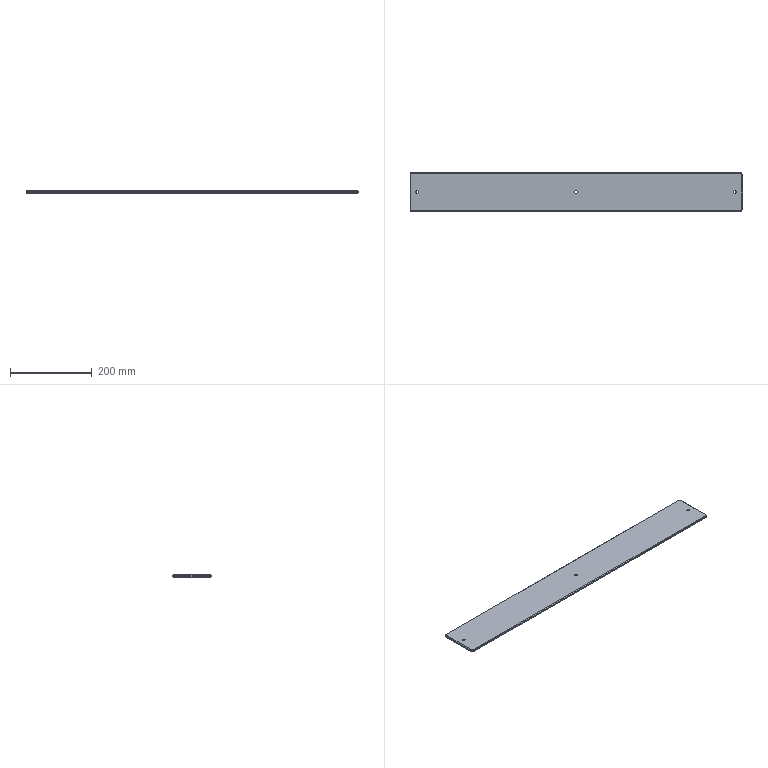Part | SolidWorks | features Chamfer 1, Extrusion 1, Fillet 1, ICE 1 | 1 solid | 32 faces | box 810 x 95 x 6 mm | volume 456909 mm3 | plane 14 | cylinder 10 | cone 8 | commonest cylinder face diameters 6.6 x6 10 x4
STEP:
#1=CARTESIAN_POINT('',(390.8,0.,0.));
#2=VERTEX_POINT('',#1);
#3=CARTESIAN_POINT('',(384.2,0.,0.));
#4=VERTEX_POINT('',#3);
#5=CARTESIAN_POINT('',(387.5,0.,0.));
#6=DIRECTION('',(0.,0.,-1.));
#7=DIRECTION('',(1.,0.,0.));
#8=AXIS2_PLACEMENT_3D('',#5,#6,#7);
#9=CIRCLE('',#8,3.3);
#10=EDGE_CURVE('',#2,#4,#9,.T.);
#11=ORIENTED_EDGE('',*,*,#10,.T.);
#12=CARTESIAN_POINT('',(384.2,0.,6.));
#13=VERTEX_POINT('',#12);
#14=CARTESIAN_POINT('',(384.2,0.,-0.001));
#15=DIRECTION('',(0.,0.,1.));
#16=VECTOR('',#15,1000.);
#17=LINE('',#14,#16);
#18=EDGE_CURVE('',#4,#13,#17,.T.);
#19=ORIENTED_EDGE('',*,*,#18,.T.);
#20=CARTESIAN_POINT('',(390.8,0.,6.));
#21=VERTEX_POINT('',#20);
#22=CARTESIAN_POINT('',(387.5,0.,6.));
#23=DIRECTION('',(0.,0.,1.));
#24=DIRECTION('',(1.,0.,0.));
#25=AXIS2_PLACEMENT_3D('',#22,#23,#24);
#26=CIRCLE('',#25,3.3);
#27=EDGE_CURVE('',#13,#21,#26,.T.);
#28=ORIENTED_EDGE('',*,*,#27,.T.);
#29=CARTESIAN_POINT('',(390.8,0.,-0.001));
#30=DIRECTION('',(0.,0.,1.));
#31=VECTOR('',#30,1000.);
#32=LINE('',#29,#31);
#33=EDGE_CURVE('',#2,#21,#32,.T.);
#34=ORIENTED_EDGE('',*,*,#33,.F.);
#35=EDGE_LOOP('',(#11,#19,#28,#34));
#36=FACE_OUTER_BOUND('',#35,.T.);
#37=CARTESIAN_POINT('',(387.5,0.,-0.001));
#38=DIRECTION('',(0.,0.,1.));
#39=DIRECTION('',(1.,0.,0.));
#40=AXIS2_PLACEMENT_3D('',#37,#38,#39);
#41=CYLINDRICAL_SURFACE('',#40,3.3);
#42=ADVANCED_FACE('',(#36),#41,.F.);
#43=CARTESIAN_POINT('',(3.3,0.,0.));
#44=VERTEX_POINT('',#43);
#45=CARTESIAN_POINT('',(-3.3,0.,0.));
#46=VERTEX_POINT('',#45);
#47=CARTESIAN_POINT('',(0.,0.,0.));
#48=DIRECTION('',(0.,0.,-1.));
#49=DIRECTION('',(1.,0.,0.));
#50=AXIS2_PLACEMENT_3D('',#47,#48,#49);
#51=CIRCLE('',#50,3.3);
#52=EDGE_CURVE('',#44,#46,#51,.T.);
#53=ORIENTED_EDGE('',*,*,#52,.T.);
#54=CARTESIAN_POINT('',(-3.3,0.,6.));
#55=VERTEX_POINT('',#54);
#56=CARTESIAN_POINT('',(-3.3,0.,-0.001));
#57=DIRECTION('',(0.,0.,1.));
#58=VECTOR('',#57,1000.);
#59=LINE('',#56,#58);
#60=EDGE_CURVE('',#46,#55,#59,.T.);
#61=ORIENTED_EDGE('',*,*,#60,.T.);
#62=CARTESIAN_POINT('',(3.3,0.,6.));
#63=VERTEX_POINT('',#62);
#64=CARTESIAN_POINT('',(0.,0.,6.));
#65=DIRECTION('',(0.,0.,1.));
#66=DIRECTION('',(1.,0.,0.));
#67=AXIS2_PLACEMENT_3D('',#64,#65,#66);
#68=CIRCLE('',#67,3.3);
#69=EDGE_CURVE('',#55,#63,#68,.T.);
#70=ORIENTED_EDGE('',*,*,#69,.T.);
#71=CARTESIAN_POINT('',(3.3,0.,-0.001));
#72=DIRECTION('',(0.,0.,1.));
#73=VECTOR('',#72,1000.);
#74=LINE('',#71,#73);
#75=EDGE_CURVE('',#44,#63,#74,.T.);
#76=ORIENTED_EDGE('',*,*,#75,.F.);
#77=EDGE_LOOP('',(#53,#61,#70,#76));
#78=FACE_OUTER_BOUND('',#77,.T.);
#79=CARTESIAN_POINT('',(0.,0.,-0.001));
#80=DIRECTION('',(0.,0.,1.));
#81=DIRECTION('',(1.,0.,0.));
#82=AXIS2_PLACEMENT_3D('',#79,#80,#81);
#83=CYLINDRICAL_SURFACE('',#82,3.3);
#84=ADVANCED_FACE('',(#78),#83,.F.);
#85=CARTESIAN_POINT('',(-384.2,0.,0.));
#86=VERTEX_POINT('',#85);
#87=CARTESIAN_POINT('',(-390.8,0.,0.));
#88=VERTEX_POINT('',#87);
#89=CARTESIAN_POINT('',(-387.5,0.,0.));
#90=DIRECTION('',(0.,0.,-1.));
#91=DIRECTION('',(1.,0.,0.));
#92=AXIS2_PLACEMENT_3D('',#89,#90,#91);
#93=CIRCLE('',#92,3.3);
#94=EDGE_CURVE('',#86,#88,#93,.T.);
#95=ORIENTED_EDGE('',*,*,#94,.T.);
#96=CARTESIAN_POINT('',(-390.8,0.,6.));
#97=VERTEX_POINT('',#96);
#98=CARTESIAN_POINT('',(-390.8,0.,-0.001));
#99=DIRECTION('',(0.,0.,1.));
#100=VECTOR('',#99,1000.);
#101=LINE('',#98,#100);
#102=EDGE_CURVE('',#88,#97,#101,.T.);
#103=ORIENTED_EDGE('',*,*,#102,.T.);
#104=CARTESIAN_POINT('',(-384.2,0.,6.));
#105=VERTEX_POINT('',#104);
#106=CARTESIAN_POINT('',(-387.5,0.,6.));
#107=DIRECTION('',(0.,0.,1.));
#108=DIRECTION('',(1.,0.,0.));
#109=AXIS2_PLACEMENT_3D('',#106,#107,#108);
#110=CIRCLE('',#109,3.3);
#111=EDGE_CURVE('',#97,#105,#110,.T.);
#112=ORIENTED_EDGE('',*,*,#111,.T.);
#113=CARTESIAN_POINT('',(-384.2,0.,-0.001));
#114=DIRECTION('',(0.,0.,1.));
#115=VECTOR('',#114,1000.);
#116=LINE('',#113,#115);
#117=EDGE_CURVE('',#86,#105,#116,.T.);
#118=ORIENTED_EDGE('',*,*,#117,.F.);
#119=EDGE_LOOP('',(#95,#103,#112,#118));
#120=FACE_OUTER_BOUND('',#119,.T.);
#121=CARTESIAN_POINT('',(-387.5,0.,-0.001));
#122=DIRECTION('',(0.,0.,1.));
#123=DIRECTION('',(1.,0.,0.));
#124=AXIS2_PLACEMENT_3D('',#121,#122,#123);
#125=CYLINDRICAL_SURFACE('',#124,3.3);
#126=ADVANCED_FACE('',(#120),#125,.F.);
#127=CARTESIAN_POINT('',(-405.,42.5,4.5));
#128=VERTEX_POINT('',#127);
#129=CARTESIAN_POINT('',(-405.,42.5,1.5));
#130=VERTEX_POINT('',#129);
#131=CARTESIAN_POINT('',(-405.,42.5,6.));
#132=DIRECTION('',(0.,0.,-1.));
#133=VECTOR('',#132,1000.);
#134=LINE('',#131,#133);
#135=EDGE_CURVE('',#128,#130,#134,.T.);
#136=ORIENTED_EDGE('',*,*,#135,.T.);
#137=CARTESIAN_POINT('',(-405.,-42.5,1.5));
#138=VERTEX_POINT('',#137);
#139=CARTESIAN_POINT('',(-405.,-47.5,1.5));
#140=DIRECTION('',(0.,-1.,0.));
#141=VECTOR('',#140,1000.);
#142=LINE('',#139,#141);
#143=EDGE_CURVE('',#130,#138,#142,.T.);
#144=ORIENTED_EDGE('',*,*,#143,.T.);
#145=CARTESIAN_POINT('',(-405.,-42.5,4.5));
#146=VERTEX_POINT('',#145);
#147=CARTESIAN_POINT('',(-405.,-42.5,6.));
#148=DIRECTION('',(0.,0.,1.));
#149=VECTOR('',#148,1000.);
#150=LINE('',#147,#149);
#151=EDGE_CURVE('',#138,#146,#150,.T.);
#152=ORIENTED_EDGE('',*,*,#151,.T.);
#153=CARTESIAN_POINT('',(-405.,42.5,4.5));
#154=DIRECTION('',(0.,1.,0.));
#155=VECTOR('',#154,1000.);
#156=LINE('',#153,#155);
#157=EDGE_CURVE('',#146,#128,#156,.T.);
#158=ORIENTED_EDGE('',*,*,#157,.T.);
#159=EDGE_LOOP('',(#136,#144,#152,#158));
#160=FACE_OUTER_BOUND('',#159,.T.);
#161=CARTESIAN_POINT('',(-405.,-47.5,6.));
#162=DIRECTION('',(1.,0.,0.));
#163=DIRECTION('',(0.,0.,-1.));
#164=AXIS2_PLACEMENT_3D('',#161,#162,#163);
#165=PLANE('',#164);
#166=ADVANCED_FACE('',(#160),#165,.F.);
#167=CARTESIAN_POINT('',(-400.,-47.5,4.5));
#168=VERTEX_POINT('',#167);
#169=CARTESIAN_POINT('',(-400.,-47.5,1.5));
#170=VERTEX_POINT('',#169);
#171=CARTESIAN_POINT('',(-400.,-47.5,6.));
#172=DIRECTION('',(0.,0.,-1.));
#173=VECTOR('',#172,1000.);
#174=LINE('',#171,#173);
#175=EDGE_CURVE('',#168,#170,#174,.T.);
#176=ORIENTED_EDGE('',*,*,#175,.T.);
#177=CARTESIAN_POINT('',(400.,-47.5,1.5));
#178=VERTEX_POINT('',#177);
#179=CARTESIAN_POINT('',(405.,-47.5,1.5));
#180=DIRECTION('',(1.,0.,0.));
#181=VECTOR('',#180,1000.);
#182=LINE('',#179,#181);
#183=EDGE_CURVE('',#170,#178,#182,.T.);
#184=ORIENTED_EDGE('',*,*,#183,.T.);
#185=CARTESIAN_POINT('',(400.,-47.5,4.5));
#186=VERTEX_POINT('',#185);
#187=CARTESIAN_POINT('',(400.,-47.5,6.));
#188=DIRECTION('',(0.,0.,1.));
#189=VECTOR('',#188,1000.);
#190=LINE('',#187,#189);
#191=EDGE_CURVE('',#178,#186,#190,.T.);
#192=ORIENTED_EDGE('',*,*,#191,.T.);
#193=CARTESIAN_POINT('',(-400.,-47.5,4.5));
#194=DIRECTION('',(-1.,0.,0.));
#195=VECTOR('',#194,1000.);
#196=LINE('',#193,#195);
#197=EDGE_CURVE('',#186,#168,#196,.T.);
#198=ORIENTED_EDGE('',*,*,#197,.T.);
#199=EDGE_LOOP('',(#176,#184,#192,#198));
#200=FACE_OUTER_BOUND('',#199,.T.);
#201=CARTESIAN_POINT('',(405.,-47.5,6.));
#202=DIRECTION('',(0.,1.,0.));
#203=DIRECTION('',(-1.,0.,0.));
#204=AXIS2_PLACEMENT_3D('',#201,#202,#203);
#205=PLANE('',#204);
#206=ADVANCED_FACE('',(#200),#205,.F.);
#207=CARTESIAN_POINT('',(405.,-42.5,4.5));
#208=VERTEX_POINT('',#207);
#209=CARTESIAN_POINT('',(405.,-42.5,1.5));
#210=VERTEX_POINT('',#209);
#211=CARTESIAN_POINT('',(405.,-42.5,6.));
#212=DIRECTION('',(0.,0.,-1.));
#213=VECTOR('',#212,1000.);
#214=LINE('',#211,#213);
#215=EDGE_CURVE('',#208,#210,#214,.T.);
#216=ORIENTED_EDGE('',*,*,#215,.T.);
#217=CARTESIAN_POINT('',(405.,42.5,1.5));
#218=VERTEX_POINT('',#217);
#219=CARTESIAN_POINT('',(405.,-47.5,1.5));
#220=DIRECTION('',(0.,1.,0.));
#221=VECTOR('',#220,1000.);
#222=LINE('',#219,#221);
#223=EDGE_CURVE('',#210,#218,#222,.T.);
#224=ORIENTED_EDGE('',*,*,#223,.T.);
#225=CARTESIAN_POINT('',(405.,42.5,4.5));
#226=VERTEX_POINT('',#225);
#227=CARTESIAN_POINT('',(405.,42.5,6.));
#228=DIRECTION('',(0.,0.,1.));
#229=VECTOR('',#228,1000.);
#230=LINE('',#227,#229);
#231=EDGE_CURVE('',#218,#226,#230,.T.);
#232=ORIENTED_EDGE('',*,*,#231,.T.);
#233=CARTESIAN_POINT('',(405.,-42.5,4.5));
#234=DIRECTION('',(0.,-1.,0.));
#235=VECTOR('',#234,1000.);
#236=LINE('',#233,#235);
#237=EDGE_CURVE('',#226,#208,#236,.T.);
#238=ORIENTED_EDGE('',*,*,#237,.T.);
#239=EDGE_LOOP('',(#216,#224,#232,#238));
#240=FACE_OUTER_BOUND('',#239,.T.);
#241=CARTESIAN_POINT('',(405.,-47.5,6.));
#242=DIRECTION('',(-1.,0.,0.));
#243=DIRECTION('',(0.,0.,1.));
#244=AXIS2_PLACEMENT_3D('',#241,#242,#243);
#245=PLANE('',#244);
#246=ADVANCED_FACE('',(#240),#245,.F.);
#247=CARTESIAN_POINT('',(400.,47.5,4.5));
#248=VERTEX_POINT('',#247);
#249=CARTESIAN_POINT('',(400.,47.5,1.5));
#250=VERTEX_POINT('',#249);
#251=CARTESIAN_POINT('',(400.,47.5,6.));
#252=DIRECTION('',(0.,0.,-1.));
#253=VECTOR('',#252,1000.);
#254=LINE('',#251,#253);
#255=EDGE_CURVE('',#248,#250,#254,.T.);
#256=ORIENTED_EDGE('',*,*,#255,.T.);
#257=CARTESIAN_POINT('',(-400.,47.5,1.5));
#258=VERTEX_POINT('',#257);
#259=CARTESIAN_POINT('',(405.,47.5,1.5));
#260=DIRECTION('',(-1.,0.,0.));
#261=VECTOR('',#260,1000.);
#262=LINE('',#259,#261);
#263=EDGE_CURVE('',#250,#258,#262,.T.);
#264=ORIENTED_EDGE('',*,*,#263,.T.);
#265=CARTESIAN_POINT('',(-400.,47.5,4.5));
#266=VERTEX_POINT('',#265);
#267=CARTESIAN_POINT('',(-400.,47.5,6.));
#268=DIRECTION('',(0.,0.,1.));
#269=VECTOR('',#268,1000.);
#270=LINE('',#267,#269);
#271=EDGE_CURVE('',#258,#266,#270,.T.);
#272=ORIENTED_EDGE('',*,*,#271,.T.);
#273=CARTESIAN_POINT('',(400.,47.5,4.5));
#274=DIRECTION('',(1.,0.,0.));
#275=VECTOR('',#274,1000.);
#276=LINE('',#273,#275);
#277=EDGE_CURVE('',#266,#248,#276,.T.);
#278=ORIENTED_EDGE('',*,*,#277,.T.);
#279=EDGE_LOOP('',(#256,#264,#272,#278));
#280=FACE_OUTER_BOUND('',#279,.T.);
#281=CARTESIAN_POINT('',(405.,47.5,6.));
#282=DIRECTION('',(0.,-1.,0.));
#283=DIRECTION('',(1.,0.,0.));
#284=AXIS2_PLACEMENT_3D('',#281,#282,#283);
#285=PLANE('',#284);
#286=ADVANCED_FACE('',(#280),#285,.F.);
#287=CARTESIAN_POINT('',(387.5,0.,6.));
#288=DIRECTION('',(0.,0.,1.));
#289=DIRECTION('',(1.,0.,0.));
#290=AXIS2_PLACEMENT_3D('',#287,#288,#289);
#291=CIRCLE('',#290,3.3);
#292=EDGE_CURVE('',#21,#13,#291,.T.);
#293=ORIENTED_EDGE('',*,*,#292,.F.);
#294=ORIENTED_EDGE('',*,*,#27,.F.);
#295=EDGE_LOOP('',(#293,#294));
#296=FACE_BOUND('',#295,.T.);
#297=CARTESIAN_POINT('',(0.,0.,6.));
#298=DIRECTION('',(0.,0.,1.));
#299=DIRECTION('',(1.,0.,0.));
#300=AXIS2_PLACEMENT_3D('',#297,#298,#299);
#301=CIRCLE('',#300,3.3);
#302=EDGE_CURVE('',#63,#55,#301,.T.);
#303=ORIENTED_EDGE('',*,*,#302,.F.);
#304=ORIENTED_EDGE('',*,*,#69,.F.);
#305=EDGE_LOOP('',(#303,#304));
#306=FACE_BOUND('',#305,.T.);
#307=CARTESIAN_POINT('',(-387.5,0.,6.));
#308=DIRECTION('',(0.,0.,1.));
#309=DIRECTION('',(1.,0.,0.));
#310=AXIS2_PLACEMENT_3D('',#307,#308,#309);
#311=CIRCLE('',#310,3.3);
#312=EDGE_CURVE('',#105,#97,#311,.T.);
#313=ORIENTED_EDGE('',*,*,#312,.F.);
#314=ORIENTED_EDGE('',*,*,#111,.F.);
#315=EDGE_LOOP('',(#313,#314));
#316=FACE_BOUND('',#315,.T.);
#317=CARTESIAN_POINT('',(-400.,-46.,6.));
#318=VERTEX_POINT('',#317);
#319=CARTESIAN_POINT('',(400.,-46.,6.));
#320=VERTEX_POINT('',#319);
#321=CARTESIAN_POINT('',(400.,-46.,6.));
#322=DIRECTION('',(1.,0.,0.));
#323=VECTOR('',#322,1000.);
#324=LINE('',#321,#323);
#325=EDGE_CURVE('',#318,#320,#324,.T.);
#326=ORIENTED_EDGE('',*,*,#325,.T.);
#327=CARTESIAN_POINT('',(403.5,-42.5,6.));
#328=VERTEX_POINT('',#327);
#329=CARTESIAN_POINT('',(400.,-42.5,6.));
#330=DIRECTION('',(0.,0.,1.));
#331=DIRECTION('',(1.,0.,0.));
#332=AXIS2_PLACEMENT_3D('',#329,#330,#331);
#333=CIRCLE('',#332,3.5);
#334=EDGE_CURVE('',#320,#328,#333,.T.);
#335=ORIENTED_EDGE('',*,*,#334,.T.);
#336=CARTESIAN_POINT('',(403.5,42.5,6.));
#337=VERTEX_POINT('',#336);
#338=CARTESIAN_POINT('',(403.5,42.5,6.));
#339=DIRECTION('',(0.,1.,0.));
#340=VECTOR('',#339,1000.);
#341=LINE('',#338,#340);
#342=EDGE_CURVE('',#328,#337,#341,.T.);
#343=ORIENTED_EDGE('',*,*,#342,.T.);
#344=CARTESIAN_POINT('',(400.,46.,6.));
#345=VERTEX_POINT('',#344);
#346=CARTESIAN_POINT('',(400.,42.5,6.));
#347=DIRECTION('',(0.,0.,1.));
#348=DIRECTION('',(1.,0.,0.));
#349=AXIS2_PLACEMENT_3D('',#346,#347,#348);
#350=CIRCLE('',#349,3.5);
#351=EDGE_CURVE('',#337,#345,#350,.T.);
#352=ORIENTED_EDGE('',*,*,#351,.T.);
#353=CARTESIAN_POINT('',(-400.,46.,6.));
#354=VERTEX_POINT('',#353);
#355=CARTESIAN_POINT('',(-400.,46.,6.));
#356=DIRECTION('',(-1.,0.,0.));
#357=VECTOR('',#356,1000.);
#358=LINE('',#355,#357);
#359=EDGE_CURVE('',#345,#354,#358,.T.);
#360=ORIENTED_EDGE('',*,*,#359,.T.);
#361=CARTESIAN_POINT('',(-403.5,42.5,6.));
#362=VERTEX_POINT('',#361);
#363=CARTESIAN_POINT('',(-400.,42.5,6.));
#364=DIRECTION('',(0.,0.,1.));
#365=DIRECTION('',(1.,0.,0.));
#366=AXIS2_PLACEMENT_3D('',#363,#364,#365);
#367=CIRCLE('',#366,3.5);
#368=EDGE_CURVE('',#354,#362,#367,.T.);
#369=ORIENTED_EDGE('',*,*,#368,.T.);
#370=CARTESIAN_POINT('',(-403.5,-42.5,6.));
#371=VERTEX_POINT('',#370);
#372=CARTESIAN_POINT('',(-403.5,-42.5,6.));
#373=DIRECTION('',(0.,-1.,0.));
#374=VECTOR('',#373,1000.);
#375=LINE('',#372,#374);
#376=EDGE_CURVE('',#362,#371,#375,.T.);
#377=ORIENTED_EDGE('',*,*,#376,.T.);
#378=CARTESIAN_POINT('',(-400.,-42.5,6.));
#379=DIRECTION('',(0.,0.,1.));
#380=DIRECTION('',(1.,0.,0.));
#381=AXIS2_PLACEMENT_3D('',#378,#379,#380);
#382=CIRCLE('',#381,3.5);
#383=EDGE_CURVE('',#371,#318,#382,.T.);
#384=ORIENTED_EDGE('',*,*,#383,.T.);
#385=EDGE_LOOP('',(#326,#335,#343,#352,#360,#369,#377,#384));
#386=FACE_OUTER_BOUND('',#385,.T.);
#387=CARTESIAN_POINT('',(0.,0.,6.));
#388=DIRECTION('',(0.,0.,1.));
#389=DIRECTION('',(1.,0.,0.));
#390=AXIS2_PLACEMENT_3D('',#387,#388,#389);
#391=PLANE('',#390);
#392=ADVANCED_FACE('',(#296,#306,#316,#386),#391,.T.);
#393=ORIENTED_EDGE('',*,*,#10,.F.);
#394=CARTESIAN_POINT('',(387.5,0.,0.));
#395=DIRECTION('',(0.,0.,-1.));
#396=DIRECTION('',(1.,0.,0.));
#397=AXIS2_PLACEMENT_3D('',#394,#395,#396);
#398=CIRCLE('',#397,3.3);
#399=EDGE_CURVE('',#4,#2,#398,.T.);
#400=ORIENTED_EDGE('',*,*,#399,.F.);
#401=EDGE_LOOP('',(#393,#400));
#402=FACE_BOUND('',#401,.T.);
#403=ORIENTED_EDGE('',*,*,#52,.F.);
#404=CARTESIAN_POINT('',(0.,0.,0.));
#405=DIRECTION('',(0.,0.,-1.));
#406=DIRECTION('',(1.,0.,0.));
#407=AXIS2_PLACEMENT_3D('',#404,#405,#406);
#408=CIRCLE('',#407,3.3);
#409=EDGE_CURVE('',#46,#44,#408,.T.);
#410=ORIENTED_EDGE('',*,*,#409,.F.);
#411=EDGE_LOOP('',(#403,#410));
#412=FACE_BOUND('',#411,.T.);
#413=ORIENTED_EDGE('',*,*,#94,.F.);
#414=CARTESIAN_POINT('',(-387.5,0.,0.));
#415=DIRECTION('',(0.,0.,-1.));
#416=DIRECTION('',(1.,0.,0.));
#417=AXIS2_PLACEMENT_3D('',#414,#415,#416);
#418=CIRCLE('',#417,3.3);
#419=EDGE_CURVE('',#88,#86,#418,.T.);
#420=ORIENTED_EDGE('',*,*,#419,.F.);
#421=EDGE_LOOP('',(#413,#420));
#422=FACE_BOUND('',#421,.T.);
#423=CARTESIAN_POINT('',(-403.5,-42.5,0.));
#424=VERTEX_POINT('',#423);
#425=CARTESIAN_POINT('',(-403.5,42.5,0.));
#426=VERTEX_POINT('',#425);
#427=CARTESIAN_POINT('',(-403.5,0.,0.));
#428=DIRECTION('',(0.,1.,0.));
#429=VECTOR('',#428,1000.);
#430=LINE('',#427,#429);
#431=EDGE_CURVE('',#424,#426,#430,.T.);
#432=ORIENTED_EDGE('',*,*,#431,.T.);
#433=CARTESIAN_POINT('',(-400.,46.,0.));
#434=VERTEX_POINT('',#433);
#435=CARTESIAN_POINT('',(-400.,42.5,0.));
#436=DIRECTION('',(0.,0.,-1.));
#437=DIRECTION('',(1.,0.,0.));
#438=AXIS2_PLACEMENT_3D('',#435,#436,#437);
#439=CIRCLE('',#438,3.5);
#440=EDGE_CURVE('',#426,#434,#439,.T.);
#441=ORIENTED_EDGE('',*,*,#440,.T.);
#442=CARTESIAN_POINT('',(400.,46.,0.));
#443=VERTEX_POINT('',#442);
#444=CARTESIAN_POINT('',(0.,46.,0.));
#445=DIRECTION('',(1.,0.,0.));
#446=VECTOR('',#445,1000.);
#447=LINE('',#444,#446);
#448=EDGE_CURVE('',#434,#443,#447,.T.);
#449=ORIENTED_EDGE('',*,*,#448,.T.);
#450=CARTESIAN_POINT('',(403.5,42.5,0.));
#451=VERTEX_POINT('',#450);
#452=CARTESIAN_POINT('',(400.,42.5,0.));
#453=DIRECTION('',(0.,0.,-1.));
#454=DIRECTION('',(1.,0.,0.));
#455=AXIS2_PLACEMENT_3D('',#452,#453,#454);
#456=CIRCLE('',#455,3.5);
#457=EDGE_CURVE('',#443,#451,#456,.T.);
#458=ORIENTED_EDGE('',*,*,#457,.T.);
#459=CARTESIAN_POINT('',(403.5,-42.5,0.));
#460=VERTEX_POINT('',#459);
#461=CARTESIAN_POINT('',(403.5,0.,0.));
#462=DIRECTION('',(0.,-1.,0.));
#463=VECTOR('',#462,1000.);
#464=LINE('',#461,#463);
#465=EDGE_CURVE('',#451,#460,#464,.T.);
#466=ORIENTED_EDGE('',*,*,#465,.T.);
#467=CARTESIAN_POINT('',(400.,-46.,0.));
#468=VERTEX_POINT('',#467);
#469=CARTESIAN_POINT('',(400.,-42.5,0.));
#470=DIRECTION('',(0.,0.,-1.));
#471=DIRECTION('',(1.,0.,0.));
#472=AXIS2_PLACEMENT_3D('',#469,#470,#471);
#473=CIRCLE('',#472,3.5);
#474=EDGE_CURVE('',#460,#468,#473,.T.);
#475=ORIENTED_EDGE('',*,*,#474,.T.);
#476=CARTESIAN_POINT('',(-400.,-46.,0.));
#477=VERTEX_POINT('',#476);
#478=CARTESIAN_POINT('',(0.,-46.,0.));
#479=DIRECTION('',(-1.,0.,0.));
#480=VECTOR('',#479,1000.);
#481=LINE('',#478,#480);
#482=EDGE_CURVE('',#468,#477,#481,.T.);
#483=ORIENTED_EDGE('',*,*,#482,.T.);
#484=CARTESIAN_POINT('',(-400.,-42.5,0.));
#485=DIRECTION('',(0.,0.,-1.));
#486=DIRECTION('',(1.,0.,0.));
#487=AXIS2_PLACEMENT_3D('',#484,#485,#486);
#488=CIRCLE('',#487,3.5);
#489=EDGE_CURVE('',#477,#424,#488,.T.);
#490=ORIENTED_EDGE('',*,*,#489,.T.);
#491=EDGE_LOOP('',(#432,#441,#449,#458,#466,#475,#483,#490));
#492=FACE_OUTER_BOUND('',#491,.T.);
#493=CARTESIAN_POINT('',(0.,0.,0.));
#494=DIRECTION('',(0.,0.,1.));
#495=DIRECTION('',(1.,0.,0.));
#496=AXIS2_PLACEMENT_3D('',#493,#494,#495);
#497=PLANE('',#496);
#498=ADVANCED_FACE('',(#402,#412,#422,#492),#497,.F.);
#499=ORIENTED_EDGE('',*,*,#231,.F.);
#500=CARTESIAN_POINT('',(400.,42.5,1.5));
#501=DIRECTION('',(0.,0.,1.));
#502=DIRECTION('',(1.,0.,0.));
#503=AXIS2_PLACEMENT_3D('',#500,#501,#502);
#504=CIRCLE('',#503,5.);
#505=EDGE_CURVE('',#218,#250,#504,.T.);
#506=ORIENTED_EDGE('',*,*,#505,.T.);
#507=ORIENTED_EDGE('',*,*,#255,.F.);
#508=CARTESIAN_POINT('',(400.,42.5,4.5));
#509=DIRECTION('',(0.,0.,-1.));
#510=DIRECTION('',(1.,0.,0.));
#511=AXIS2_PLACEMENT_3D('',#508,#509,#510);
#512=CIRCLE('',#511,5.);
#513=EDGE_CURVE('',#248,#226,#512,.T.);
#514=ORIENTED_EDGE('',*,*,#513,.T.);
#515=EDGE_LOOP('',(#499,#506,#507,#514));
#516=FACE_OUTER_BOUND('',#515,.T.);
#517=CARTESIAN_POINT('',(400.,42.5,6.));
#518=DIRECTION('',(0.,0.,-1.));
#519=DIRECTION('',(-1.,0.,0.));
#520=AXIS2_PLACEMENT_3D('',#517,#518,#519);
#521=CYLINDRICAL_SURFACE('',#520,5.);
#522=ADVANCED_FACE('',(#516),#521,.T.);
#523=ORIENTED_EDGE('',*,*,#191,.F.);
#524=CARTESIAN_POINT('',(400.,-42.5,1.5));
#525=DIRECTION('',(0.,0.,1.));
#526=DIRECTION('',(1.,0.,0.));
#527=AXIS2_PLACEMENT_3D('',#524,#525,#526);
#528=CIRCLE('',#527,5.);
#529=EDGE_CURVE('',#178,#210,#528,.T.);
#530=ORIENTED_EDGE('',*,*,#529,.T.);
#531=ORIENTED_EDGE('',*,*,#215,.F.);
#532=CARTESIAN_POINT('',(400.,-42.5,4.5));
#533=DIRECTION('',(0.,0.,-1.));
#534=DIRECTION('',(1.,0.,0.));
#535=AXIS2_PLACEMENT_3D('',#532,#533,#534);
#536=CIRCLE('',#535,5.);
#537=EDGE_CURVE('',#208,#186,#536,.T.);
#538=ORIENTED_EDGE('',*,*,#537,.T.);
#539=EDGE_LOOP('',(#523,#530,#531,#538));
#540=FACE_OUTER_BOUND('',#539,.T.);
#541=CARTESIAN_POINT('',(400.,-42.5,6.));
#542=DIRECTION('',(0.,0.,-1.));
#543=DIRECTION('',(-1.,0.,0.));
#544=AXIS2_PLACEMENT_3D('',#541,#542,#543);
#545=CYLINDRICAL_SURFACE('',#544,5.);
#546=ADVANCED_FACE('',(#540),#545,.T.);
#547=ORIENTED_EDGE('',*,*,#151,.F.);
#548=CARTESIAN_POINT('',(-400.,-42.5,1.5));
#549=DIRECTION('',(0.,0.,1.));
#550=DIRECTION('',(1.,0.,0.));
#551=AXIS2_PLACEMENT_3D('',#548,#549,#550);
#552=CIRCLE('',#551,5.);
#553=EDGE_CURVE('',#138,#170,#552,.T.);
#554=ORIENTED_EDGE('',*,*,#553,.T.);
#555=ORIENTED_EDGE('',*,*,#175,.F.);
#556=CARTESIAN_POINT('',(-400.,-42.5,4.5));
#557=DIRECTION('',(0.,0.,-1.));
#558=DIRECTION('',(1.,0.,0.));
#559=AXIS2_PLACEMENT_3D('',#556,#557,#558);
#560=CIRCLE('',#559,5.);
#561=EDGE_CURVE('',#168,#146,#560,.T.);
#562=ORIENTED_EDGE('',*,*,#561,.T.);
#563=EDGE_LOOP('',(#547,#554,#555,#562));
#564=FACE_OUTER_BOUND('',#563,.T.);
#565=CARTESIAN_POINT('',(-400.,-42.5,6.));
#566=DIRECTION('',(0.,0.,-1.));
#567=DIRECTION('',(-1.,0.,0.));
#568=AXIS2_PLACEMENT_3D('',#565,#566,#567);
#569=CYLINDRICAL_SURFACE('',#568,5.);
#570=ADVANCED_FACE('',(#564),#569,.T.);
#571=ORIENTED_EDGE('',*,*,#271,.F.);
#572=CARTESIAN_POINT('',(-400.,42.5,1.5));
#573=DIRECTION('',(0.,0.,1.));
#574=DIRECTION('',(1.,0.,0.));
#575=AXIS2_PLACEMENT_3D('',#572,#573,#574);
#576=CIRCLE('',#575,5.);
#577=EDGE_CURVE('',#258,#130,#576,.T.);
#578=ORIENTED_EDGE('',*,*,#577,.T.);
#579=ORIENTED_EDGE('',*,*,#135,.F.);
#580=CARTESIAN_POINT('',(-400.,42.5,4.5));
#581=DIRECTION('',(0.,0.,-1.));
#582=DIRECTION('',(1.,0.,0.));
#583=AXIS2_PLACEMENT_3D('',#580,#581,#582);
#584=CIRCLE('',#583,5.);
#585=EDGE_CURVE('',#128,#266,#584,.T.);
#586=ORIENTED_EDGE('',*,*,#585,.T.);
#587=EDGE_LOOP('',(#571,#578,#579,#586));
#588=FACE_OUTER_BOUND('',#587,.T.);
#589=CARTESIAN_POINT('',(-400.,42.5,6.));
#590=DIRECTION('',(0.,0.,-1.));
#591=DIRECTION('',(-1.,0.,0.));
#592=AXIS2_PLACEMENT_3D('',#589,#590,#591);
#593=CYLINDRICAL_SURFACE('',#592,5.);
#594=ADVANCED_FACE('',(#588),#593,.T.);
#595=CARTESIAN_POINT('',(405.,-42.5,1.5));
#596=DIRECTION('',(-0.7071,0.,-0.7071));
#597=VECTOR('',#596,1000.);
#598=LINE('',#595,#597);
#599=EDGE_CURVE('',#210,#460,#598,.T.);
#600=ORIENTED_EDGE('',*,*,#599,.F.);
#601=ORIENTED_EDGE('',*,*,#529,.F.);
#602=CARTESIAN_POINT('',(400.,-46.,0.));
#603=DIRECTION('',(0.,-0.7071,0.7071));
#604=VECTOR('',#603,1000.);
#605=LINE('',#602,#604);
#606=EDGE_CURVE('',#468,#178,#605,.T.);
#607=ORIENTED_EDGE('',*,*,#606,.F.);
#608=ORIENTED_EDGE('',*,*,#474,.F.);
#609=EDGE_LOOP('',(#600,#601,#607,#608));
#610=FACE_OUTER_BOUND('',#609,.T.);
#611=CARTESIAN_POINT('',(400.,-42.5,0.));
#612=DIRECTION('',(0.,0.,1.));
#613=DIRECTION('',(1.,0.,0.));
#614=AXIS2_PLACEMENT_3D('',#611,#612,#613);
#615=CONICAL_SURFACE('',#614,3.5,0.7854);
#616=ADVANCED_FACE('',(#610),#615,.T.);
#617=ORIENTED_EDGE('',*,*,#606,.T.);
#618=ORIENTED_EDGE('',*,*,#183,.F.);
#619=CARTESIAN_POINT('',(-400.,-46.,0.));
#620=DIRECTION('',(0.,-0.7071,0.7071));
#621=VECTOR('',#620,1000.);
#622=LINE('',#619,#621);
#623=EDGE_CURVE('',#477,#170,#622,.T.);
#624=ORIENTED_EDGE('',*,*,#623,.F.);
#625=ORIENTED_EDGE('',*,*,#482,.F.);
#626=EDGE_LOOP('',(#617,#618,#624,#625));
#627=FACE_OUTER_BOUND('',#626,.T.);
#628=CARTESIAN_POINT('',(405.,-47.5,1.5));
#629=DIRECTION('',(0.,0.7071,0.7071));
#630=DIRECTION('',(1.,0.,0.));
#631=AXIS2_PLACEMENT_3D('',#628,#629,#630);
#632=PLANE('',#631);
#633=ADVANCED_FACE('',(#627),#632,.F.);
#634=ORIENTED_EDGE('',*,*,#599,.T.);
#635=ORIENTED_EDGE('',*,*,#465,.F.);
#636=CARTESIAN_POINT('',(405.,42.5,1.5));
#637=DIRECTION('',(-0.7071,0.,-0.7071));
#638=VECTOR('',#637,1000.);
#639=LINE('',#636,#638);
#640=EDGE_CURVE('',#218,#451,#639,.T.);
#641=ORIENTED_EDGE('',*,*,#640,.F.);
#642=ORIENTED_EDGE('',*,*,#223,.F.);
#643=EDGE_LOOP('',(#634,#635,#641,#642));
#644=FACE_OUTER_BOUND('',#643,.T.);
#645=CARTESIAN_POINT('',(405.,-47.5,1.5));
#646=DIRECTION('',(-0.7071,0.,0.7071));
#647=DIRECTION('',(0.,1.,0.));
#648=AXIS2_PLACEMENT_3D('',#645,#646,#647);
#649=PLANE('',#648);
#650=ADVANCED_FACE('',(#644),#649,.F.);
#651=ORIENTED_EDGE('',*,*,#623,.T.);
#652=ORIENTED_EDGE('',*,*,#553,.F.);
#653=CARTESIAN_POINT('',(-403.5,-42.5,0.));
#654=DIRECTION('',(-0.7071,0.,0.7071));
#655=VECTOR('',#654,1000.);
#656=LINE('',#653,#655);
#657=EDGE_CURVE('',#424,#138,#656,.T.);
#658=ORIENTED_EDGE('',*,*,#657,.F.);
#659=ORIENTED_EDGE('',*,*,#489,.F.);
#660=EDGE_LOOP('',(#651,#652,#658,#659));
#661=FACE_OUTER_BOUND('',#660,.T.);
#662=CARTESIAN_POINT('',(-400.,-42.5,0.));
#663=DIRECTION('',(0.,0.,1.));
#664=DIRECTION('',(1.,0.,0.));
#665=AXIS2_PLACEMENT_3D('',#662,#663,#664);
#666=CONICAL_SURFACE('',#665,3.5,0.7854);
#667=ADVANCED_FACE('',(#661),#666,.T.);
#668=ORIENTED_EDGE('',*,*,#640,.T.);
#669=ORIENTED_EDGE('',*,*,#457,.F.);
#670=CARTESIAN_POINT('',(400.,47.5,1.5));
#671=DIRECTION('',(0.,-0.7071,-0.7071));
#672=VECTOR('',#671,1000.);
#673=LINE('',#670,#672);
#674=EDGE_CURVE('',#250,#443,#673,.T.);
#675=ORIENTED_EDGE('',*,*,#674,.F.);
#676=ORIENTED_EDGE('',*,*,#505,.F.);
#677=EDGE_LOOP('',(#668,#669,#675,#676));
#678=FACE_OUTER_BOUND('',#677,.T.);
#679=CARTESIAN_POINT('',(400.,42.5,0.));
#680=DIRECTION('',(0.,0.,1.));
#681=DIRECTION('',(1.,0.,0.));
#682=AXIS2_PLACEMENT_3D('',#679,#680,#681);
#683=CONICAL_SURFACE('',#682,3.5,0.7854);
#684=ADVANCED_FACE('',(#678),#683,.T.);
#685=ORIENTED_EDGE('',*,*,#657,.T.);
#686=ORIENTED_EDGE('',*,*,#143,.F.);
#687=CARTESIAN_POINT('',(-403.5,42.5,0.));
#688=DIRECTION('',(-0.7071,0.,0.7071));
#689=VECTOR('',#688,1000.);
#690=LINE('',#687,#689);
#691=EDGE_CURVE('',#426,#130,#690,.T.);
#692=ORIENTED_EDGE('',*,*,#691,.F.);
#693=ORIENTED_EDGE('',*,*,#431,.F.);
#694=EDGE_LOOP('',(#685,#686,#692,#693));
#695=FACE_OUTER_BOUND('',#694,.T.);
#696=CARTESIAN_POINT('',(-405.,-47.5,1.5));
#697=DIRECTION('',(0.7071,0.,0.7071));
#698=DIRECTION('',(0.,-1.,0.));
#699=AXIS2_PLACEMENT_3D('',#696,#697,#698);
#700=PLANE('',#699);
#701=ADVANCED_FACE('',(#695),#700,.F.);
#702=ORIENTED_EDGE('',*,*,#674,.T.);
#703=ORIENTED_EDGE('',*,*,#448,.F.);
#704=CARTESIAN_POINT('',(-400.,47.5,1.5));
#705=DIRECTION('',(0.,-0.7071,-0.7071));
#706=VECTOR('',#705,1000.);
#707=LINE('',#704,#706);
#708=EDGE_CURVE('',#258,#434,#707,.T.);
#709=ORIENTED_EDGE('',*,*,#708,.F.);
#710=ORIENTED_EDGE('',*,*,#263,.F.);
#711=EDGE_LOOP('',(#702,#703,#709,#710));
#712=FACE_OUTER_BOUND('',#711,.T.);
#713=CARTESIAN_POINT('',(405.,47.5,1.5));
#714=DIRECTION('',(0.,-0.7071,0.7071));
#715=DIRECTION('',(-1.,0.,0.));
#716=AXIS2_PLACEMENT_3D('',#713,#714,#715);
#717=PLANE('',#716);
#718=ADVANCED_FACE('',(#712),#717,.F.);
#719=ORIENTED_EDGE('',*,*,#691,.T.);
#720=ORIENTED_EDGE('',*,*,#577,.F.);
#721=ORIENTED_EDGE('',*,*,#708,.T.);
#722=ORIENTED_EDGE('',*,*,#440,.F.);
#723=EDGE_LOOP('',(#719,#720,#721,#722));
#724=FACE_OUTER_BOUND('',#723,.T.);
#725=CARTESIAN_POINT('',(-400.,42.5,0.));
#726=DIRECTION('',(0.,0.,1.));
#727=DIRECTION('',(1.,0.,0.));
#728=AXIS2_PLACEMENT_3D('',#725,#726,#727);
#729=CONICAL_SURFACE('',#728,3.5,0.7854);
#730=ADVANCED_FACE('',(#724),#729,.T.);
#731=CARTESIAN_POINT('',(-400.,47.5,4.5));
#732=DIRECTION('',(0.,-0.7071,0.7071));
#733=VECTOR('',#732,1000.);
#734=LINE('',#731,#733);
#735=EDGE_CURVE('',#266,#354,#734,.T.);
#736=ORIENTED_EDGE('',*,*,#735,.F.);
#737=ORIENTED_EDGE('',*,*,#585,.F.);
#738=CARTESIAN_POINT('',(-403.5,42.5,6.));
#739=DIRECTION('',(-0.7071,0.,-0.7071));
#740=VECTOR('',#739,1000.);
#741=LINE('',#738,#740);
#742=EDGE_CURVE('',#362,#128,#741,.T.);
#743=ORIENTED_EDGE('',*,*,#742,.F.);
#744=ORIENTED_EDGE('',*,*,#368,.F.);
#745=EDGE_LOOP('',(#736,#737,#743,#744));
#746=FACE_OUTER_BOUND('',#745,.T.);
#747=CARTESIAN_POINT('',(-400.,42.5,6.));
#748=DIRECTION('',(0.,0.,-1.));
#749=DIRECTION('',(-1.,0.,0.));
#750=AXIS2_PLACEMENT_3D('',#747,#748,#749);
#751=CONICAL_SURFACE('',#750,3.5,0.7854);
#752=ADVANCED_FACE('',(#746),#751,.T.);
#753=ORIENTED_EDGE('',*,*,#742,.T.);
#754=ORIENTED_EDGE('',*,*,#157,.F.);
#755=CARTESIAN_POINT('',(-403.5,-42.5,6.));
#756=DIRECTION('',(-0.7071,0.,-0.7071));
#757=VECTOR('',#756,1000.);
#758=LINE('',#755,#757);
#759=EDGE_CURVE('',#371,#146,#758,.T.);
#760=ORIENTED_EDGE('',*,*,#759,.F.);
#761=ORIENTED_EDGE('',*,*,#376,.F.);
#762=EDGE_LOOP('',(#753,#754,#760,#761));
#763=FACE_OUTER_BOUND('',#762,.T.);
#764=CARTESIAN_POINT('',(-403.5,0.,6.));
#765=DIRECTION('',(-0.7071,0.,0.7071));
#766=DIRECTION('',(0.,1.,0.));
#767=AXIS2_PLACEMENT_3D('',#764,#765,#766);
#768=PLANE('',#767);
#769=ADVANCED_FACE('',(#763),#768,.T.);
#770=ORIENTED_EDGE('',*,*,#735,.T.);
#771=ORIENTED_EDGE('',*,*,#359,.F.);
#772=CARTESIAN_POINT('',(400.,47.5,4.5));
#773=DIRECTION('',(0.,-0.7071,0.7071));
#774=VECTOR('',#773,1000.);
#775=LINE('',#772,#774);
#776=EDGE_CURVE('',#248,#345,#775,.T.);
#777=ORIENTED_EDGE('',*,*,#776,.F.);
#778=ORIENTED_EDGE('',*,*,#277,.F.);
#779=EDGE_LOOP('',(#770,#771,#777,#778));
#780=FACE_OUTER_BOUND('',#779,.T.);
#781=CARTESIAN_POINT('',(0.,46.,6.));
#782=DIRECTION('',(0.,0.7071,0.7071));
#783=DIRECTION('',(1.,0.,0.));
#784=AXIS2_PLACEMENT_3D('',#781,#782,#783);
#785=PLANE('',#784);
#786=ADVANCED_FACE('',(#780),#785,.T.);
#787=ORIENTED_EDGE('',*,*,#759,.T.);
#788=ORIENTED_EDGE('',*,*,#561,.F.);
#789=CARTESIAN_POINT('',(-400.,-46.,6.));
#790=DIRECTION('',(0.,-0.7071,-0.7071));
#791=VECTOR('',#790,1000.);
#792=LINE('',#789,#791);
#793=EDGE_CURVE('',#318,#168,#792,.T.);
#794=ORIENTED_EDGE('',*,*,#793,.F.);
#795=ORIENTED_EDGE('',*,*,#383,.F.);
#796=EDGE_LOOP('',(#787,#788,#794,#795));
#797=FACE_OUTER_BOUND('',#796,.T.);
#798=CARTESIAN_POINT('',(-400.,-42.5,6.));
#799=DIRECTION('',(0.,0.,-1.));
#800=DIRECTION('',(-1.,0.,0.));
#801=AXIS2_PLACEMENT_3D('',#798,#799,#800);
#802=CONICAL_SURFACE('',#801,3.5,0.7854);
#803=ADVANCED_FACE('',(#797),#802,.T.);
#804=ORIENTED_EDGE('',*,*,#776,.T.);
#805=ORIENTED_EDGE('',*,*,#351,.F.);
#806=CARTESIAN_POINT('',(405.,42.5,4.5));
#807=DIRECTION('',(-0.7071,0.,0.7071));
#808=VECTOR('',#807,1000.);
#809=LINE('',#806,#808);
#810=EDGE_CURVE('',#226,#337,#809,.T.);
#811=ORIENTED_EDGE('',*,*,#810,.F.);
#812=ORIENTED_EDGE('',*,*,#513,.F.);
#813=EDGE_LOOP('',(#804,#805,#811,#812));
#814=FACE_OUTER_BOUND('',#813,.T.);
#815=CARTESIAN_POINT('',(400.,42.5,6.));
#816=DIRECTION('',(0.,0.,-1.));
#817=DIRECTION('',(-1.,0.,0.));
#818=AXIS2_PLACEMENT_3D('',#815,#816,#817);
#819=CONICAL_SURFACE('',#818,3.5,0.7854);
#820=ADVANCED_FACE('',(#814),#819,.T.);
#821=ORIENTED_EDGE('',*,*,#793,.T.);
#822=ORIENTED_EDGE('',*,*,#197,.F.);
#823=CARTESIAN_POINT('',(400.,-46.,6.));
#824=DIRECTION('',(0.,-0.7071,-0.7071));
#825=VECTOR('',#824,1000.);
#826=LINE('',#823,#825);
#827=EDGE_CURVE('',#320,#186,#826,.T.);
#828=ORIENTED_EDGE('',*,*,#827,.F.);
#829=ORIENTED_EDGE('',*,*,#325,.F.);
#830=EDGE_LOOP('',(#821,#822,#828,#829));
#831=FACE_OUTER_BOUND('',#830,.T.);
#832=CARTESIAN_POINT('',(0.,-46.,6.));
#833=DIRECTION('',(0.,-0.7071,0.7071));
#834=DIRECTION('',(-1.,0.,0.));
#835=AXIS2_PLACEMENT_3D('',#832,#833,#834);
#836=PLANE('',#835);
#837=ADVANCED_FACE('',(#831),#836,.T.);
#838=ORIENTED_EDGE('',*,*,#810,.T.);
#839=ORIENTED_EDGE('',*,*,#342,.F.);
#840=CARTESIAN_POINT('',(405.,-42.5,4.5));
#841=DIRECTION('',(-0.7071,0.,0.7071));
#842=VECTOR('',#841,1000.);
#843=LINE('',#840,#842);
#844=EDGE_CURVE('',#208,#328,#843,.T.);
#845=ORIENTED_EDGE('',*,*,#844,.F.);
#846=ORIENTED_EDGE('',*,*,#237,.F.);
#847=EDGE_LOOP('',(#838,#839,#845,#846));
#848=FACE_OUTER_BOUND('',#847,.T.);
#849=CARTESIAN_POINT('',(403.5,0.,6.));
#850=DIRECTION('',(0.7071,0.,0.7071));
#851=DIRECTION('',(0.,-1.,0.));
#852=AXIS2_PLACEMENT_3D('',#849,#850,#851);
#853=PLANE('',#852);
#854=ADVANCED_FACE('',(#848),#853,.T.);
#855=ORIENTED_EDGE('',*,*,#827,.T.);
#856=ORIENTED_EDGE('',*,*,#537,.F.);
#857=ORIENTED_EDGE('',*,*,#844,.T.);
#858=ORIENTED_EDGE('',*,*,#334,.F.);
#859=EDGE_LOOP('',(#855,#856,#857,#858));
#860=FACE_OUTER_BOUND('',#859,.T.);
#861=CARTESIAN_POINT('',(400.,-42.5,6.));
#862=DIRECTION('',(0.,0.,-1.));
#863=DIRECTION('',(-1.,0.,0.));
#864=AXIS2_PLACEMENT_3D('',#861,#862,#863);
#865=CONICAL_SURFACE('',#864,3.5,0.7854);
#866=ADVANCED_FACE('',(#860),#865,.T.);
#867=ORIENTED_EDGE('',*,*,#102,.F.);
#868=ORIENTED_EDGE('',*,*,#419,.T.);
#869=ORIENTED_EDGE('',*,*,#117,.T.);
#870=ORIENTED_EDGE('',*,*,#312,.T.);
#871=EDGE_LOOP('',(#867,#868,#869,#870));
#872=FACE_OUTER_BOUND('',#871,.T.);
#873=CARTESIAN_POINT('',(-387.5,0.,-0.001));
#874=DIRECTION('',(0.,0.,1.));
#875=DIRECTION('',(1.,0.,0.));
#876=AXIS2_PLACEMENT_3D('',#873,#874,#875);
#877=CYLINDRICAL_SURFACE('',#876,3.3);
#878=ADVANCED_FACE('',(#872),#877,.F.);
#879=ORIENTED_EDGE('',*,*,#60,.F.);
#880=ORIENTED_EDGE('',*,*,#409,.T.);
#881=ORIENTED_EDGE('',*,*,#75,.T.);
#882=ORIENTED_EDGE('',*,*,#302,.T.);
#883=EDGE_LOOP('',(#879,#880,#881,#882));
#884=FACE_OUTER_BOUND('',#883,.T.);
#885=CARTESIAN_POINT('',(0.,0.,-0.001));
#886=DIRECTION('',(0.,0.,1.));
#887=DIRECTION('',(1.,0.,0.));
#888=AXIS2_PLACEMENT_3D('',#885,#886,#887);
#889=CYLINDRICAL_SURFACE('',#888,3.3);
#890=ADVANCED_FACE('',(#884),#889,.F.);
#891=ORIENTED_EDGE('',*,*,#18,.F.);
#892=ORIENTED_EDGE('',*,*,#399,.T.);
#893=ORIENTED_EDGE('',*,*,#33,.T.);
#894=ORIENTED_EDGE('',*,*,#292,.T.);
#895=EDGE_LOOP('',(#891,#892,#893,#894));
#896=FACE_OUTER_BOUND('',#895,.T.);
#897=CARTESIAN_POINT('',(387.5,0.,-0.001));
#898=DIRECTION('',(0.,0.,1.));
#899=DIRECTION('',(1.,0.,0.));
#900=AXIS2_PLACEMENT_3D('',#897,#898,#899);
#901=CYLINDRICAL_SURFACE('',#900,3.3);
#902=ADVANCED_FACE('',(#896),#901,.F.);
#903=CLOSED_SHELL('',(#42,#84,#126,#166,#206,#246,#286,#392,#498,#522,#546,#570,#594,#616,#633,#650,#667,#684,#701,#718,#730,#752,#769,#786,#803,#820,#837,#854,#866,#878,#890,#902));
#904=MANIFOLD_SOLID_BREP('',#903);
#905=CARTESIAN_POINT('',(0.,0.,0.));
#906=DIRECTION('',(0.,0.,1.));
#907=DIRECTION('',(1.,0.,0.));
#908=AXIS2_PLACEMENT_3D('',#905,#906,#907);
#909=(LENGTH_UNIT()NAMED_UNIT(*)SI_UNIT(.MILLI.,.METRE.));
#910=UNCERTAINTY_MEASURE_WITH_UNIT(LENGTH_MEASURE(0.00001),#909,'','');
#911=(NAMED_UNIT(*)PLANE_ANGLE_UNIT()SI_UNIT($,.RADIAN.));
#912=(NAMED_UNIT(*)SI_UNIT($,.STERADIAN.)SOLID_ANGLE_UNIT());
#913=(GEOMETRIC_REPRESENTATION_CONTEXT(3)GLOBAL_UNCERTAINTY_ASSIGNED_CONTEXT((#910))GLOBAL_UNIT_ASSIGNED_CONTEXT((#909,#911,#912))REPRESENTATION_CONTEXT('',''));
#914=ADVANCED_BREP_SHAPE_REPRESENTATION('',(#904,#908),#913);